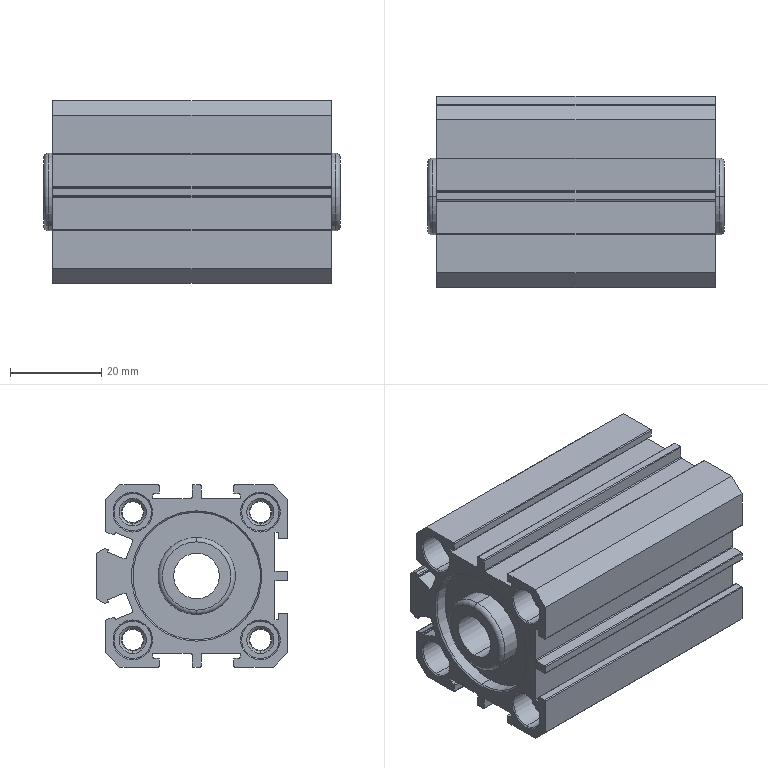Part | STEP file | 001-008-_SDAJS-25x30_30b | 1 solid | 245 faces | box 65 x 42 x 40 mm | volume 54492 mm3 | cylinder 111 | plane 86 | cone 44 | torus 4 | commonest cylinder face diameters 0.4 x46 4.917 x16 8.2 x16 4.6 x8 0.8 x7 4.134 x4